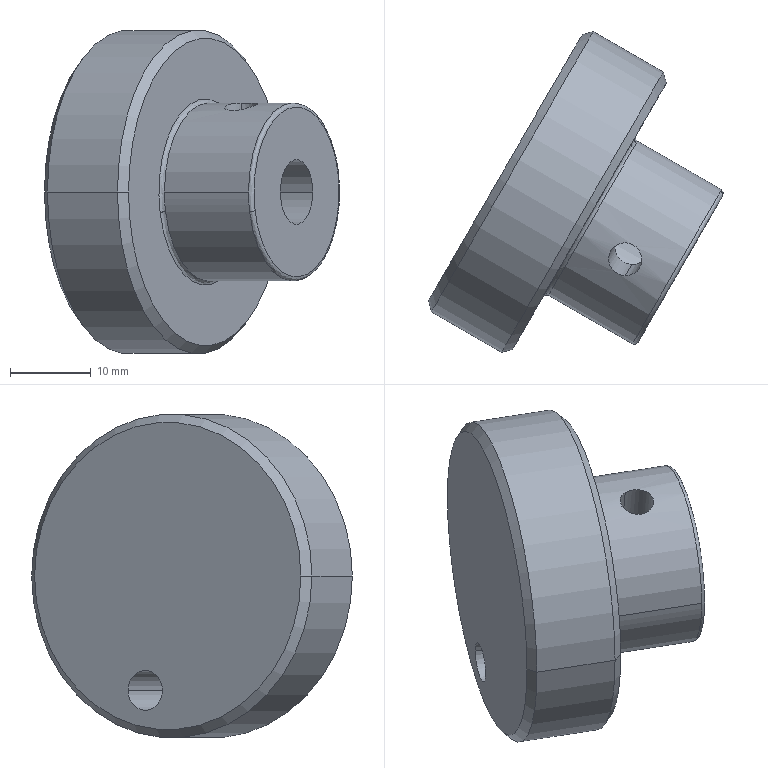Part | SolidWorks | features BaseBody 1 | 1 solid | 26 faces | box 36.468 x 39.641 x 40 mm | volume 18831 mm3 | cylinder 10 | cone 8 | spline 4 | plane 4 | commonest cylinder face diameters 4.134 x2 4.917 x2 8 x2 22 x2 40 x2
STEP:
#1=CARTESIAN_POINT('',(-287.209,1830.124,-1175.566));
#2=VERTEX_POINT('',#1);
#3=CARTESIAN_POINT('',(-298.072,1811.308,-1178.));
#4=VERTEX_POINT('',#3);
#5=CARTESIAN_POINT('',(-292.572,1820.834,-1178.));
#6=DIRECTION('',(0.866,-0.5,0.));
#7=DIRECTION('',(-0.4876,-0.8446,-0.2213));
#8=AXIS2_PLACEMENT_3D('',#5,#6,#7);
#9=CIRCLE('',#8,11.);
#10=EDGE_CURVE('',#2,#4,#9,.T.);
#11=ORIENTED_EDGE('',*,*,#10,.F.);
#12=CARTESIAN_POINT('',(-287.398,1830.796,-1175.455));
#13=VERTEX_POINT('',#12);
#14=CARTESIAN_POINT('',(-286.965,1830.546,-1175.455));
#15=DIRECTION('',(0.1106,0.1916,-0.9752));
#16=DIRECTION('',(0.4876,0.8446,0.2213));
#17=AXIS2_PLACEMENT_3D('',#14,#15,#16);
#18=CIRCLE('',#17,0.5);
#19=EDGE_CURVE('',#2,#13,#18,.T.);
#20=ORIENTED_EDGE('',*,*,#19,.T.);
#21=CARTESIAN_POINT('',(-298.613,1811.372,-1180.545));
#22=VERTEX_POINT('',#21);
#23=CARTESIAN_POINT('',(-287.398,1830.796,-1175.455));
#24=CARTESIAN_POINT('',(-288.143,1829.506,-1168.886));
#25=CARTESIAN_POINT('',(-290.993,1824.57,-1165.294));
#26=CARTESIAN_POINT('',(-294.278,1818.88,-1166.785));
#27=CARTESIAN_POINT('',(-297.562,1813.191,-1168.276));
#28=CARTESIAN_POINT('',(-299.358,1810.081,-1173.975));
#29=CARTESIAN_POINT('',(-298.613,1811.372,-1180.545));
#30=(BOUNDED_CURVE()B_SPLINE_CURVE(3,(#23,#24,#25,#26,#27,#28,#29),.UNSPECIFIED.,.F.,.F.)B_SPLINE_CURVE_WITH_KNOTS((4,3,4),(0.,0.5,1.),.UNSPECIFIED.)CURVE()GEOMETRIC_REPRESENTATION_ITEM()RATIONAL_B_SPLINE_CURVE((1.,0.8047,0.8047,1.,0.8047,0.8047,1.))REPRESENTATION_ITEM(''));
#31=EDGE_CURVE('',#13,#22,#30,.T.);
#32=ORIENTED_EDGE('',*,*,#31,.T.);
#33=CARTESIAN_POINT('',(-297.936,1811.544,-1180.434));
#34=VERTEX_POINT('',#33);
#35=CARTESIAN_POINT('',(-298.18,1811.122,-1180.545));
#36=DIRECTION('',(-0.1106,-0.1916,0.9752));
#37=DIRECTION('',(-0.4876,-0.8446,-0.2213));
#38=AXIS2_PLACEMENT_3D('',#35,#36,#37);
#39=CIRCLE('',#38,0.5);
#40=EDGE_CURVE('',#34,#22,#39,.T.);
#41=ORIENTED_EDGE('',*,*,#40,.F.);
#42=CARTESIAN_POINT('',(-292.572,1820.834,-1178.));
#43=DIRECTION('',(0.866,-0.5,0.));
#44=DIRECTION('',(-0.4876,-0.8446,-0.2213));
#45=AXIS2_PLACEMENT_3D('',#42,#43,#44);
#46=CIRCLE('',#45,11.);
#47=EDGE_CURVE('',#4,#34,#46,.T.);
#48=ORIENTED_EDGE('',*,*,#47,.F.);
#49=EDGE_LOOP('',(#11,#20,#32,#41,#48));
#50=FACE_OUTER_BOUND('',#49,.T.);
#51=CARTESIAN_POINT('',(-297.936,1811.544,-1180.434));
#52=CARTESIAN_POINT('',(-298.649,1810.309,-1174.15));
#53=CARTESIAN_POINT('',(-296.931,1813.284,-1168.698));
#54=CARTESIAN_POINT('',(-293.789,1818.726,-1167.273));
#55=CARTESIAN_POINT('',(-290.647,1824.168,-1165.847));
#56=CARTESIAN_POINT('',(-287.922,1828.889,-1169.282));
#57=CARTESIAN_POINT('',(-287.209,1830.124,-1175.566));
#58=CARTESIAN_POINT('',(-298.19,1811.69,-1180.434));
#59=CARTESIAN_POINT('',(-298.903,1810.456,-1174.15));
#60=CARTESIAN_POINT('',(-297.185,1813.431,-1168.698));
#61=CARTESIAN_POINT('',(-294.043,1818.873,-1167.273));
#62=CARTESIAN_POINT('',(-290.901,1824.315,-1165.847));
#63=CARTESIAN_POINT('',(-288.175,1829.036,-1169.282));
#64=CARTESIAN_POINT('',(-287.462,1830.271,-1175.566));
#65=CARTESIAN_POINT('',(-298.47,1811.619,-1180.48));
#66=CARTESIAN_POINT('',(-299.196,1810.361,-1174.078));
#67=CARTESIAN_POINT('',(-297.446,1813.392,-1168.523));
#68=CARTESIAN_POINT('',(-294.245,1818.936,-1167.071));
#69=CARTESIAN_POINT('',(-291.044,1824.481,-1165.618));
#70=CARTESIAN_POINT('',(-288.267,1829.291,-1169.118));
#71=CARTESIAN_POINT('',(-287.541,1830.549,-1175.52));
#72=CARTESIAN_POINT('',(-298.613,1811.372,-1180.545));
#73=CARTESIAN_POINT('',(-299.358,1810.081,-1173.975));
#74=CARTESIAN_POINT('',(-297.562,1813.191,-1168.276));
#75=CARTESIAN_POINT('',(-294.278,1818.88,-1166.785));
#76=CARTESIAN_POINT('',(-290.993,1824.57,-1165.294));
#77=CARTESIAN_POINT('',(-288.143,1829.506,-1168.886));
#78=CARTESIAN_POINT('',(-287.398,1830.796,-1175.455));
#79=(BOUNDED_SURFACE()B_SPLINE_SURFACE(3,3,((#51,#52,#53,#54,#55,#56,#57),(#58,#59,#60,#61,#62,#63,#64),(#65,#66,#67,#68,#69,#70,#71),(#72,#73,#74,#75,#76,#77,#78)),.UNSPECIFIED.,.F.,.F.,.F.)B_SPLINE_SURFACE_WITH_KNOTS((4,4),(4,3,4),(0.,1.),(0.,0.5,1.),.UNSPECIFIED.)GEOMETRIC_REPRESENTATION_ITEM()RATIONAL_B_SPLINE_SURFACE(((1.,0.8047,0.8047,1.,0.8047,0.8047,1.),(0.8047,0.6476,0.6476,0.8047,0.6476,0.6476,0.8047),(0.8047,0.6476,0.6476,0.8047,0.6476,0.6476,0.8047),(1.,0.8047,0.8047,1.,0.8047,0.8047,1.)))REPRESENTATION_ITEM('')SURFACE());
#80=ADVANCED_FACE('',(#50),#79,.F.);
#81=CARTESIAN_POINT('',(-276.816,1824.124,-1175.566));
#82=VERTEX_POINT('',#81);
#83=CARTESIAN_POINT('',(-276.68,1824.36,-1178.));
#84=VERTEX_POINT('',#83);
#85=CARTESIAN_POINT('',(-282.18,1814.834,-1178.));
#86=DIRECTION('',(-0.866,0.5,0.));
#87=DIRECTION('',(-0.5,-0.866,0.));
#88=AXIS2_PLACEMENT_3D('',#85,#86,#87);
#89=CIRCLE('',#88,11.);
#90=EDGE_CURVE('',#82,#84,#89,.T.);
#91=ORIENTED_EDGE('',*,*,#90,.F.);
#92=CARTESIAN_POINT('',(-276.627,1823.452,-1175.677));
#93=VERTEX_POINT('',#92);
#94=CARTESIAN_POINT('',(-277.06,1823.702,-1175.677));
#95=DIRECTION('',(0.1106,0.1916,-0.9752));
#96=DIRECTION('',(0.4876,0.8446,0.2213));
#97=AXIS2_PLACEMENT_3D('',#94,#95,#96);
#98=CIRCLE('',#97,0.5);
#99=EDGE_CURVE('',#82,#93,#98,.T.);
#100=ORIENTED_EDGE('',*,*,#99,.T.);
#101=CARTESIAN_POINT('',(-286.867,1805.716,-1180.323));
#102=VERTEX_POINT('',#101);
#103=CARTESIAN_POINT('',(-276.627,1823.452,-1175.677));
#104=CARTESIAN_POINT('',(-274.304,1827.476,-1196.156));
#105=CARTESIAN_POINT('',(-284.544,1809.74,-1200.803));
#106=CARTESIAN_POINT('',(-286.867,1805.716,-1180.323));
#107=(BOUNDED_CURVE()B_SPLINE_CURVE(3,(#103,#104,#105,#106),.UNSPECIFIED.,.F.,.F.)B_SPLINE_CURVE_WITH_KNOTS((4,4),(0.,1.),.UNSPECIFIED.)CURVE()GEOMETRIC_REPRESENTATION_ITEM()RATIONAL_B_SPLINE_CURVE((1.,0.3333,0.3333,1.))REPRESENTATION_ITEM(''));
#108=EDGE_CURVE('',#93,#102,#107,.T.);
#109=ORIENTED_EDGE('',*,*,#108,.T.);
#110=CARTESIAN_POINT('',(-287.544,1805.544,-1180.434));
#111=VERTEX_POINT('',#110);
#112=CARTESIAN_POINT('',(-287.3,1805.966,-1180.323));
#113=DIRECTION('',(-0.1106,-0.1916,0.9752));
#114=DIRECTION('',(-0.4876,-0.8446,-0.2213));
#115=AXIS2_PLACEMENT_3D('',#112,#113,#114);
#116=CIRCLE('',#115,0.5);
#117=EDGE_CURVE('',#111,#102,#116,.T.);
#118=ORIENTED_EDGE('',*,*,#117,.F.);
#119=CARTESIAN_POINT('',(-282.18,1814.834,-1178.));
#120=DIRECTION('',(-0.866,0.5,0.));
#121=DIRECTION('',(-0.5,-0.866,0.));
#122=AXIS2_PLACEMENT_3D('',#119,#120,#121);
#123=CIRCLE('',#122,11.);
#124=EDGE_CURVE('',#84,#111,#123,.T.);
#125=ORIENTED_EDGE('',*,*,#124,.F.);
#126=EDGE_LOOP('',(#91,#100,#109,#118,#125));
#127=FACE_OUTER_BOUND('',#126,.T.);
#128=CARTESIAN_POINT('',(-276.816,1824.124,-1175.566));
#129=CARTESIAN_POINT('',(-274.382,1828.34,-1197.021));
#130=CARTESIAN_POINT('',(-285.11,1809.76,-1201.889));
#131=CARTESIAN_POINT('',(-287.544,1805.544,-1180.434));
#132=CARTESIAN_POINT('',(-276.563,1823.978,-1175.566));
#133=CARTESIAN_POINT('',(-274.129,1828.193,-1197.021));
#134=CARTESIAN_POINT('',(-284.856,1809.613,-1201.889));
#135=CARTESIAN_POINT('',(-287.29,1805.397,-1180.434));
#136=CARTESIAN_POINT('',(-276.484,1823.699,-1175.612));
#137=CARTESIAN_POINT('',(-274.096,1827.836,-1196.663));
#138=CARTESIAN_POINT('',(-284.622,1809.605,-1201.439));
#139=CARTESIAN_POINT('',(-287.01,1805.469,-1180.388));
#140=CARTESIAN_POINT('',(-276.627,1823.452,-1175.677));
#141=CARTESIAN_POINT('',(-274.304,1827.476,-1196.156));
#142=CARTESIAN_POINT('',(-284.544,1809.74,-1200.803));
#143=CARTESIAN_POINT('',(-286.867,1805.716,-1180.323));
#144=(BOUNDED_SURFACE()B_SPLINE_SURFACE(3,3,((#128,#129,#130,#131),(#132,#133,#134,#135),(#136,#137,#138,#139),(#140,#141,#142,#143)),.UNSPECIFIED.,.F.,.F.,.F.)B_SPLINE_SURFACE_WITH_KNOTS((4,4),(4,4),(0.,1.),(0.,1.),.UNSPECIFIED.)GEOMETRIC_REPRESENTATION_ITEM()RATIONAL_B_SPLINE_SURFACE(((1.,0.3333,0.3333,1.),(0.8047,0.2682,0.2682,0.8047),(0.8047,0.2682,0.2682,0.8047),(1.,0.3333,0.3333,1.)))REPRESENTATION_ITEM('')SURFACE());
#145=ADVANCED_FACE('',(#127),#144,.T.);
#146=CARTESIAN_POINT('',(-292.77,1827.492,-1192.141));
#147=VERTEX_POINT('',#146);
#148=CARTESIAN_POINT('',(-295.229,1823.233,-1192.141));
#149=VERTEX_POINT('',#148);
#150=CARTESIAN_POINT('',(-293.999,1825.363,-1192.141));
#151=DIRECTION('',(-0.866,0.5,0.));
#152=DIRECTION('',(-0.5,-0.866,0.));
#153=AXIS2_PLACEMENT_3D('',#150,#151,#152);
#154=CIRCLE('',#153,2.459);
#155=EDGE_CURVE('',#147,#149,#154,.T.);
#156=ORIENTED_EDGE('',*,*,#155,.F.);
#157=CARTESIAN_POINT('',(-300.564,1831.992,-1192.141));
#158=VERTEX_POINT('',#157);
#159=CARTESIAN_POINT('',(-300.564,1831.992,-1192.141));
#160=DIRECTION('',(-0.866,0.5,0.));
#161=VECTOR('',#160,1000.);
#162=LINE('',#159,#161);
#163=EDGE_CURVE('',#147,#158,#162,.T.);
#164=ORIENTED_EDGE('',*,*,#163,.T.);
#165=CARTESIAN_POINT('',(-303.023,1827.733,-1192.141));
#166=VERTEX_POINT('',#165);
#167=CARTESIAN_POINT('',(-301.794,1829.863,-1192.141));
#168=DIRECTION('',(-0.866,0.5,0.));
#169=DIRECTION('',(-0.5,-0.866,0.));
#170=AXIS2_PLACEMENT_3D('',#167,#168,#169);
#171=CIRCLE('',#170,2.459);
#172=EDGE_CURVE('',#158,#166,#171,.T.);
#173=ORIENTED_EDGE('',*,*,#172,.T.);
#174=CARTESIAN_POINT('',(-303.023,1827.733,-1192.141));
#175=DIRECTION('',(-0.866,0.5,0.));
#176=VECTOR('',#175,1000.);
#177=LINE('',#174,#176);
#178=EDGE_CURVE('',#149,#166,#177,.T.);
#179=ORIENTED_EDGE('',*,*,#178,.F.);
#180=EDGE_LOOP('',(#156,#164,#173,#179));
#181=FACE_OUTER_BOUND('',#180,.T.);
#182=CARTESIAN_POINT('',(-301.794,1829.863,-1192.141));
#183=DIRECTION('',(-0.866,0.5,0.));
#184=DIRECTION('',(-0.5,-0.866,0.));
#185=AXIS2_PLACEMENT_3D('',#182,#183,#184);
#186=CYLINDRICAL_SURFACE('',#185,2.459);
#187=ADVANCED_FACE('',(#181),#186,.F.);
#188=CARTESIAN_POINT('',(-293.898,1843.538,-1178.));
#189=VERTEX_POINT('',#188);
#190=CARTESIAN_POINT('',(-312.898,1810.63,-1178.));
#191=VERTEX_POINT('',#190);
#192=CARTESIAN_POINT('',(-303.398,1827.084,-1178.));
#193=DIRECTION('',(0.866,-0.5,0.));
#194=DIRECTION('',(0.5,0.866,0.));
#195=AXIS2_PLACEMENT_3D('',#192,#193,#194);
#196=CIRCLE('',#195,19.);
#197=EDGE_CURVE('',#189,#191,#196,.T.);
#198=ORIENTED_EDGE('',*,*,#197,.T.);
#199=CARTESIAN_POINT('',(-312.532,1809.264,-1178.));
#200=VERTEX_POINT('',#199);
#201=CARTESIAN_POINT('',(-312.532,1809.264,-1178.));
#202=DIRECTION('',(0.2588,-0.9659,0.));
#203=VECTOR('',#202,1000.);
#204=LINE('',#201,#203);
#205=EDGE_CURVE('',#191,#200,#204,.T.);
#206=ORIENTED_EDGE('',*,*,#205,.T.);
#207=CARTESIAN_POINT('',(-292.532,1843.905,-1178.));
#208=VERTEX_POINT('',#207);
#209=CARTESIAN_POINT('',(-302.532,1826.584,-1178.));
#210=DIRECTION('',(-0.866,0.5,0.));
#211=DIRECTION('',(0.4876,0.8446,0.2213));
#212=AXIS2_PLACEMENT_3D('',#209,#210,#211);
#213=CIRCLE('',#212,20.);
#214=EDGE_CURVE('',#200,#208,#213,.T.);
#215=ORIENTED_EDGE('',*,*,#214,.T.);
#216=CARTESIAN_POINT('',(-292.532,1843.905,-1178.));
#217=DIRECTION('',(0.9659,0.2588,0.));
#218=VECTOR('',#217,1000.);
#219=LINE('',#216,#218);
#220=EDGE_CURVE('',#189,#208,#219,.T.);
#221=ORIENTED_EDGE('',*,*,#220,.F.);
#222=EDGE_LOOP('',(#198,#206,#215,#221));
#223=FACE_OUTER_BOUND('',#222,.T.);
#224=CARTESIAN_POINT('',(-302.532,1826.584,-1178.));
#225=DIRECTION('',(0.866,-0.5,0.));
#226=DIRECTION('',(0.5,0.866,0.));
#227=AXIS2_PLACEMENT_3D('',#224,#225,#226);
#228=CONICAL_SURFACE('',#227,20.,0.7854);
#229=ADVANCED_FACE('',(#223),#228,.T.);
#230=CARTESIAN_POINT('',(-292.587,1826.809,-1192.141));
#231=VERTEX_POINT('',#230);
#232=CARTESIAN_POINT('',(-294.546,1823.416,-1192.141));
#233=VERTEX_POINT('',#232);
#234=CARTESIAN_POINT('',(-293.566,1825.113,-1192.141));
#235=DIRECTION('',(-0.866,0.5,0.));
#236=DIRECTION('',(-0.5,-0.866,0.));
#237=AXIS2_PLACEMENT_3D('',#234,#235,#236);
#238=CIRCLE('',#237,1.959);
#239=EDGE_CURVE('',#231,#233,#238,.T.);
#240=ORIENTED_EDGE('',*,*,#239,.F.);
#241=CARTESIAN_POINT('',(-292.77,1827.492,-1192.141));
#242=DIRECTION('',(-0.2588,0.9659,0.));
#243=VECTOR('',#242,1000.);
#244=LINE('',#241,#243);
#245=EDGE_CURVE('',#231,#147,#244,.T.);
#246=ORIENTED_EDGE('',*,*,#245,.T.);
#247=ORIENTED_EDGE('',*,*,#155,.T.);
#248=CARTESIAN_POINT('',(-295.229,1823.233,-1192.141));
#249=DIRECTION('',(-0.9659,-0.2588,0.));
#250=VECTOR('',#249,1000.);
#251=LINE('',#248,#250);
#252=EDGE_CURVE('',#233,#149,#251,.T.);
#253=ORIENTED_EDGE('',*,*,#252,.F.);
#254=EDGE_LOOP('',(#240,#246,#247,#253));
#255=FACE_OUTER_BOUND('',#254,.T.);
#256=CARTESIAN_POINT('',(-293.999,1825.363,-1192.141));
#257=DIRECTION('',(-0.866,0.5,0.));
#258=DIRECTION('',(-0.5,-0.866,0.));
#259=AXIS2_PLACEMENT_3D('',#256,#257,#258);
#260=CONICAL_SURFACE('',#259,2.458,0.7854);
#261=ADVANCED_FACE('',(#255),#260,.F.);
#262=CARTESIAN_POINT('',(-303.871,1804.264,-1178.));
#263=VERTEX_POINT('',#262);
#264=CARTESIAN_POINT('',(-283.871,1838.905,-1178.));
#265=VERTEX_POINT('',#264);
#266=CARTESIAN_POINT('',(-293.871,1821.584,-1178.));
#267=DIRECTION('',(-0.866,0.5,0.));
#268=DIRECTION('',(-0.5,-0.866,0.));
#269=AXIS2_PLACEMENT_3D('',#266,#267,#268);
#270=CIRCLE('',#269,20.);
#271=EDGE_CURVE('',#263,#265,#270,.T.);
#272=ORIENTED_EDGE('',*,*,#271,.T.);
#273=CARTESIAN_POINT('',(-293.398,1844.405,-1178.));
#274=DIRECTION('',(-0.866,0.5,0.));
#275=VECTOR('',#274,1000.);
#276=LINE('',#273,#275);
#277=EDGE_CURVE('',#265,#208,#276,.T.);
#278=ORIENTED_EDGE('',*,*,#277,.T.);
#279=ORIENTED_EDGE('',*,*,#214,.F.);
#280=CARTESIAN_POINT('',(-313.398,1809.764,-1178.));
#281=DIRECTION('',(-0.866,0.5,0.));
#282=VECTOR('',#281,1000.);
#283=LINE('',#280,#282);
#284=EDGE_CURVE('',#263,#200,#283,.T.);
#285=ORIENTED_EDGE('',*,*,#284,.F.);
#286=EDGE_LOOP('',(#272,#278,#279,#285));
#287=FACE_OUTER_BOUND('',#286,.T.);
#288=CARTESIAN_POINT('',(-303.398,1827.084,-1178.));
#289=DIRECTION('',(-0.866,0.5,0.));
#290=DIRECTION('',(-0.5,-0.866,0.));
#291=AXIS2_PLACEMENT_3D('',#288,#289,#290);
#292=CYLINDRICAL_SURFACE('',#291,20.);
#293=ADVANCED_FACE('',(#287),#292,.T.);
#294=CARTESIAN_POINT('',(-302.505,1804.63,-1178.));
#295=VERTEX_POINT('',#294);
#296=CARTESIAN_POINT('',(-283.505,1837.538,-1178.));
#297=VERTEX_POINT('',#296);
#298=CARTESIAN_POINT('',(-293.005,1821.084,-1178.));
#299=DIRECTION('',(-0.866,0.5,0.));
#300=DIRECTION('',(-0.5,-0.866,0.));
#301=AXIS2_PLACEMENT_3D('',#298,#299,#300);
#302=CIRCLE('',#301,19.);
#303=EDGE_CURVE('',#295,#297,#302,.T.);
#304=ORIENTED_EDGE('',*,*,#303,.T.);
#305=CARTESIAN_POINT('',(-283.871,1838.905,-1178.));
#306=DIRECTION('',(-0.2588,0.9659,0.));
#307=VECTOR('',#306,1000.);
#308=LINE('',#305,#307);
#309=EDGE_CURVE('',#297,#265,#308,.T.);
#310=ORIENTED_EDGE('',*,*,#309,.T.);
#311=ORIENTED_EDGE('',*,*,#271,.F.);
#312=CARTESIAN_POINT('',(-303.871,1804.264,-1178.));
#313=DIRECTION('',(-0.9659,-0.2588,0.));
#314=VECTOR('',#313,1000.);
#315=LINE('',#312,#314);
#316=EDGE_CURVE('',#295,#263,#315,.T.);
#317=ORIENTED_EDGE('',*,*,#316,.F.);
#318=EDGE_LOOP('',(#304,#310,#311,#317));
#319=FACE_OUTER_BOUND('',#318,.T.);
#320=CARTESIAN_POINT('',(-293.871,1821.584,-1178.));
#321=DIRECTION('',(-0.866,0.5,0.));
#322=DIRECTION('',(-0.5,-0.866,0.));
#323=AXIS2_PLACEMENT_3D('',#320,#321,#322);
#324=CONICAL_SURFACE('',#323,20.,0.7854);
#325=ADVANCED_FACE('',(#319),#324,.T.);
#326=CARTESIAN_POINT('',(-288.577,1813.726,-1167.816));
#327=VERTEX_POINT('',#326);
#328=CARTESIAN_POINT('',(-288.577,1817.783,-1167.019));
#329=VERTEX_POINT('',#328);
#330=CARTESIAN_POINT('',(-288.577,1813.726,-1167.816));
#331=CARTESIAN_POINT('',(-288.71,1813.731,-1167.841));
#332=CARTESIAN_POINT('',(-288.845,1813.749,-1167.863));
#333=CARTESIAN_POINT('',(-289.105,1813.81,-1167.896));
#334=CARTESIAN_POINT('',(-289.233,1813.852,-1167.908));
#335=CARTESIAN_POINT('',(-289.484,1813.961,-1167.922));
#336=CARTESIAN_POINT('',(-289.604,1814.028,-1167.923));
#337=CARTESIAN_POINT('',(-289.828,1814.18,-1167.914));
#338=CARTESIAN_POINT('',(-289.932,1814.265,-1167.905));
#339=CARTESIAN_POINT('',(-290.124,1814.455,-1167.875));
#340=CARTESIAN_POINT('',(-290.211,1814.56,-1167.855));
#341=CARTESIAN_POINT('',(-290.362,1814.779,-1167.808));
#342=CARTESIAN_POINT('',(-290.426,1814.895,-1167.78));
#343=CARTESIAN_POINT('',(-290.532,1815.139,-1167.719));
#344=CARTESIAN_POINT('',(-290.572,1815.264,-1167.685));
#345=CARTESIAN_POINT('',(-290.627,1815.519,-1167.616));
#346=CARTESIAN_POINT('',(-290.641,1815.651,-1167.579));
#347=CARTESIAN_POINT('',(-290.643,1815.912,-1167.505));
#348=CARTESIAN_POINT('',(-290.631,1816.041,-1167.469));
#349=CARTESIAN_POINT('',(-290.58,1816.297,-1167.397));
#350=CARTESIAN_POINT('',(-290.541,1816.425,-1167.362));
#351=CARTESIAN_POINT('',(-290.388,1816.787,-1167.264));
#352=CARTESIAN_POINT('',(-290.233,1817.011,-1167.207));
#353=CARTESIAN_POINT('',(-289.851,1817.381,-1167.118));
#354=CARTESIAN_POINT('',(-289.619,1817.531,-1167.085));
#355=CARTESIAN_POINT('',(-289.244,1817.682,-1167.051));
#356=CARTESIAN_POINT('',(-289.112,1817.721,-1167.042));
#357=CARTESIAN_POINT('',(-288.847,1817.771,-1167.028));
#358=CARTESIAN_POINT('',(-288.713,1817.784,-1167.023));
#359=CARTESIAN_POINT('',(-288.577,1817.783,-1167.019));
#360=B_SPLINE_CURVE_WITH_KNOTS('',3,(#330,#331,#332,#333,#334,#335,#336,#337,#338,#339,#340,#341,#342,#343,#344,#345,#346,#347,#348,#349,#350,#351,#352,#353,#354,#355,#356,#357,#358,#359),.UNSPECIFIED.,.F.,.F.,(4,2,2,2,2,2,2,2,2,2,2,2,2,2,4),(0.0119,0.0123,0.01271,0.01311,0.01352,0.01392,0.01432,0.01473,0.01513,0.01554,0.01594,0.01675,0.01756,0.01797,0.01837),.UNSPECIFIED.);
#361=EDGE_CURVE('',#327,#329,#360,.T.);
#362=ORIENTED_EDGE('',*,*,#361,.T.);
#363=CARTESIAN_POINT('',(-288.577,1817.783,-1167.019));
#364=CARTESIAN_POINT('',(-288.441,1817.782,-1167.015));
#365=CARTESIAN_POINT('',(-288.304,1817.768,-1167.012));
#366=CARTESIAN_POINT('',(-288.04,1817.713,-1167.009));
#367=CARTESIAN_POINT('',(-287.911,1817.673,-1167.008));
#368=CARTESIAN_POINT('',(-287.659,1817.566,-1167.006));
#369=CARTESIAN_POINT('',(-287.538,1817.5,-1167.006));
#370=CARTESIAN_POINT('',(-287.315,1817.346,-1167.007));
#371=CARTESIAN_POINT('',(-287.212,1817.259,-1167.008));
#372=CARTESIAN_POINT('',(-287.024,1817.064,-1167.011));
#373=CARTESIAN_POINT('',(-286.938,1816.956,-1167.013));
#374=CARTESIAN_POINT('',(-286.793,1816.729,-1167.02));
#375=CARTESIAN_POINT('',(-286.731,1816.609,-1167.024));
#376=CARTESIAN_POINT('',(-286.63,1816.354,-1167.037));
#377=CARTESIAN_POINT('',(-286.593,1816.225,-1167.045));
#378=CARTESIAN_POINT('',(-286.544,1815.96,-1167.066));
#379=CARTESIAN_POINT('',(-286.532,1815.824,-1167.079));
#380=CARTESIAN_POINT('',(-286.535,1815.554,-1167.11));
#381=CARTESIAN_POINT('',(-286.549,1815.421,-1167.128));
#382=CARTESIAN_POINT('',(-286.603,1815.159,-1167.17));
#383=CARTESIAN_POINT('',(-286.644,1815.03,-1167.194));
#384=CARTESIAN_POINT('',(-286.799,1814.664,-1167.275));
#385=CARTESIAN_POINT('',(-286.953,1814.442,-1167.34));
#386=CARTESIAN_POINT('',(-287.329,1814.081,-1167.481));
#387=CARTESIAN_POINT('',(-287.556,1813.94,-1167.557));
#388=CARTESIAN_POINT('',(-287.923,1813.804,-1167.663));
#389=CARTESIAN_POINT('',(-288.052,1813.77,-1167.698));
#390=CARTESIAN_POINT('',(-288.312,1813.729,-1167.762));
#391=CARTESIAN_POINT('',(-288.443,1813.721,-1167.791));
#392=CARTESIAN_POINT('',(-288.577,1813.726,-1167.816));
#393=B_SPLINE_CURVE_WITH_KNOTS('',3,(#363,#364,#365,#366,#367,#368,#369,#370,#371,#372,#373,#374,#375,#376,#377,#378,#379,#380,#381,#382,#383,#384,#385,#386,#387,#388,#389,#390,#391,#392),.UNSPECIFIED.,.F.,.F.,(4,2,2,2,2,2,2,2,2,2,2,2,2,2,4),(0.005421,0.005826,0.006231,0.006635,0.00704,0.007445,0.00785,0.008254,0.008659,0.009064,0.009468,0.01028,0.01109,0.01149,0.0119),.UNSPECIFIED.);
#394=EDGE_CURVE('',#329,#327,#393,.T.);
#395=ORIENTED_EDGE('',*,*,#394,.T.);
#396=EDGE_LOOP('',(#362,#395));
#397=FACE_BOUND('',#396,.T.);
#398=CARTESIAN_POINT('',(-287.68,1805.308,-1178.));
#399=VERTEX_POINT('',#398);
#400=CARTESIAN_POINT('',(-282.18,1814.834,-1178.));
#401=DIRECTION('',(-0.866,0.5,0.));
#402=DIRECTION('',(-0.5,-0.866,0.));
#403=AXIS2_PLACEMENT_3D('',#400,#401,#402);
#404=CIRCLE('',#403,11.);
#405=EDGE_CURVE('',#399,#82,#404,.T.);
#406=ORIENTED_EDGE('',*,*,#405,.T.);
#407=ORIENTED_EDGE('',*,*,#90,.T.);
#408=CARTESIAN_POINT('',(-287.072,1830.36,-1178.));
#409=VERTEX_POINT('',#408);
#410=CARTESIAN_POINT('',(-297.898,1836.61,-1178.));
#411=DIRECTION('',(-0.866,0.5,0.));
#412=VECTOR('',#411,1000.);
#413=LINE('',#410,#412);
#414=EDGE_CURVE('',#84,#409,#413,.T.);
#415=ORIENTED_EDGE('',*,*,#414,.T.);
#416=CARTESIAN_POINT('',(-292.572,1820.834,-1178.));
#417=DIRECTION('',(0.866,-0.5,0.));
#418=DIRECTION('',(-0.4876,-0.8446,-0.2213));
#419=AXIS2_PLACEMENT_3D('',#416,#417,#418);
#420=CIRCLE('',#419,11.);
#421=EDGE_CURVE('',#409,#2,#420,.T.);
#422=ORIENTED_EDGE('',*,*,#421,.T.);
#423=ORIENTED_EDGE('',*,*,#10,.T.);
#424=CARTESIAN_POINT('',(-308.898,1817.558,-1178.));
#425=DIRECTION('',(-0.866,0.5,0.));
#426=VECTOR('',#425,1000.);
#427=LINE('',#424,#426);
#428=EDGE_CURVE('',#399,#4,#427,.T.);
#429=ORIENTED_EDGE('',*,*,#428,.F.);
#430=EDGE_LOOP('',(#406,#407,#415,#422,#423,#429));
#431=FACE_OUTER_BOUND('',#430,.T.);
#432=CARTESIAN_POINT('',(-303.398,1827.084,-1178.));
#433=DIRECTION('',(-0.866,0.5,0.));
#434=DIRECTION('',(-0.5,-0.866,0.));
#435=AXIS2_PLACEMENT_3D('',#432,#433,#434);
#436=CYLINDRICAL_SURFACE('',#435,11.);
#437=ADVANCED_FACE('',(#397,#431),#436,.T.);
#438=CARTESIAN_POINT('',(-287.771,1819.178,-1174.118));
#439=VERTEX_POINT('',#438);
#440=CARTESIAN_POINT('',(-287.771,1815.121,-1174.916));
#441=VERTEX_POINT('',#440);
#442=CARTESIAN_POINT('',(-287.771,1819.178,-1174.118));
#443=CARTESIAN_POINT('',(-287.908,1819.174,-1174.101));
#444=CARTESIAN_POINT('',(-288.045,1819.157,-1174.082));
#445=CARTESIAN_POINT('',(-288.312,1819.099,-1174.048));
#446=CARTESIAN_POINT('',(-288.442,1819.057,-1174.033));
#447=CARTESIAN_POINT('',(-288.696,1818.95,-1174.01));
#448=CARTESIAN_POINT('',(-288.819,1818.885,-1174.003));
#449=CARTESIAN_POINT('',(-289.047,1818.734,-1173.999));
#450=CARTESIAN_POINT('',(-289.155,1818.649,-1174.002));
#451=CARTESIAN_POINT('',(-289.354,1818.456,-1174.023));
#452=CARTESIAN_POINT('',(-289.443,1818.353,-1174.041));
#453=CARTESIAN_POINT('',(-289.596,1818.131,-1174.09));
#454=CARTESIAN_POINT('',(-289.662,1818.012,-1174.122));
#455=CARTESIAN_POINT('',(-289.766,1817.768,-1174.199));
#456=CARTESIAN_POINT('',(-289.804,1817.644,-1174.243));
#457=CARTESIAN_POINT('',(-289.852,1817.39,-1174.342));
#458=CARTESIAN_POINT('',(-289.862,1817.262,-1174.396));
#459=CARTESIAN_POINT('',(-289.855,1817.01,-1174.507));
#460=CARTESIAN_POINT('',(-289.838,1816.885,-1174.565));
#461=CARTESIAN_POINT('',(-289.779,1816.641,-1174.681));
#462=CARTESIAN_POINT('',(-289.737,1816.523,-1174.737));
#463=CARTESIAN_POINT('',(-289.629,1816.293,-1174.845));
#464=CARTESIAN_POINT('',(-289.563,1816.181,-1174.897));
#465=CARTESIAN_POINT('',(-289.41,1815.971,-1174.985));
#466=CARTESIAN_POINT('',(-289.323,1815.872,-1175.023));
#467=CARTESIAN_POINT('',(-289.031,1815.592,-1175.112));
#468=CARTESIAN_POINT('',(-288.794,1815.432,-1175.132));
#469=CARTESIAN_POINT('',(-288.295,1815.208,-1175.08));
#470=CARTESIAN_POINT('',(-288.03,1815.14,-1175.009));
#471=CARTESIAN_POINT('',(-287.771,1815.121,-1174.916));
#472=B_SPLINE_CURVE_WITH_KNOTS('',3,(#442,#443,#444,#445,#446,#447,#448,#449,#450,#451,#452,#453,#454,#455,#456,#457,#458,#459,#460,#461,#462,#463,#464,#465,#466,#467,#468,#469,#470,#471),.UNSPECIFIED.,.F.,.F.,(4,2,2,2,2,2,2,2,2,2,2,2,2,2,4),(0.001068,0.001479,0.00189,0.002301,0.002713,0.003124,0.003535,0.003946,0.004357,0.004768,0.005179,0.005591,0.006002,0.006824,0.007646),.UNSPECIFIED.);
#473=EDGE_CURVE('',#439,#441,#472,.T.);
#474=ORIENTED_EDGE('',*,*,#473,.F.);
#475=CARTESIAN_POINT('',(-288.593,1817.754,-1166.874));
#476=DIRECTION('',(-0.1106,-0.1916,0.9752));
#477=VECTOR('',#476,1000.);
#478=LINE('',#475,#477);
#479=EDGE_CURVE('',#439,#329,#478,.T.);
#480=ORIENTED_EDGE('',*,*,#479,.T.);
#481=ORIENTED_EDGE('',*,*,#361,.F.);
#482=CARTESIAN_POINT('',(-288.593,1813.698,-1167.671));
#483=DIRECTION('',(-0.1106,-0.1916,0.9752));
#484=VECTOR('',#483,1000.);
#485=LINE('',#482,#484);
#486=EDGE_CURVE('',#441,#327,#485,.T.);
#487=ORIENTED_EDGE('',*,*,#486,.F.);
#488=EDGE_LOOP('',(#474,#480,#481,#487));
#489=FACE_OUTER_BOUND('',#488,.T.);
#490=CARTESIAN_POINT('',(-288.593,1815.726,-1167.273));
#491=DIRECTION('',(-0.1106,-0.1916,0.9752));
#492=DIRECTION('',(0.,-0.9812,-0.1928));
#493=AXIS2_PLACEMENT_3D('',#490,#491,#492);
#494=CYLINDRICAL_SURFACE('',#493,2.067);
#495=ADVANCED_FACE('',(#489),#494,.F.);
#496=CARTESIAN_POINT('',(-296.737,1818.62,-1178.));
#497=VERTEX_POINT('',#496);
#498=CARTESIAN_POINT('',(-292.737,1825.548,-1178.));
#499=VERTEX_POINT('',#498);
#500=CARTESIAN_POINT('',(-294.737,1822.084,-1178.));
#501=DIRECTION('',(0.866,-0.5,0.));
#502=DIRECTION('',(0.5,0.866,0.));
#503=AXIS2_PLACEMENT_3D('',#500,#501,#502);
#504=CIRCLE('',#503,4.);
#505=EDGE_CURVE('',#497,#499,#504,.T.);
#506=ORIENTED_EDGE('',*,*,#505,.F.);
#507=CARTESIAN_POINT('',(-283.747,1811.12,-1178.));
#508=VERTEX_POINT('',#507);
#509=CARTESIAN_POINT('',(-283.747,1811.12,-1178.));
#510=DIRECTION('',(0.866,-0.5,0.));
#511=VECTOR('',#510,1000.);
#512=LINE('',#509,#511);
#513=EDGE_CURVE('',#497,#508,#512,.T.);
#514=ORIENTED_EDGE('',*,*,#513,.T.);
#515=CARTESIAN_POINT('',(-279.747,1818.048,-1178.));
#516=VERTEX_POINT('',#515);
#517=CARTESIAN_POINT('',(-281.747,1814.584,-1178.));
#518=DIRECTION('',(-0.866,0.5,0.));
#519=DIRECTION('',(0.5,0.866,0.));
#520=AXIS2_PLACEMENT_3D('',#517,#518,#519);
#521=CIRCLE('',#520,4.);
#522=EDGE_CURVE('',#516,#508,#521,.T.);
#523=ORIENTED_EDGE('',*,*,#522,.F.);
#524=CARTESIAN_POINT('',(-279.747,1818.048,-1178.));
#525=DIRECTION('',(0.866,-0.5,0.));
#526=VECTOR('',#525,1000.);
#527=LINE('',#524,#526);
#528=EDGE_CURVE('',#499,#516,#527,.T.);
#529=ORIENTED_EDGE('',*,*,#528,.F.);
#530=EDGE_LOOP('',(#506,#514,#523,#529));
#531=FACE_OUTER_BOUND('',#530,.T.);
#532=CARTESIAN_POINT('',(-281.747,1814.584,-1178.));
#533=DIRECTION('',(0.866,-0.5,0.));
#534=DIRECTION('',(0.5,0.866,0.));
#535=AXIS2_PLACEMENT_3D('',#532,#533,#534);
#536=CYLINDRICAL_SURFACE('',#535,4.);
#537=ADVANCED_FACE('',(#531),#536,.F.);
#538=CARTESIAN_POINT('',(-296.819,1823.286,-1178.));
#539=VERTEX_POINT('',#538);
#540=CARTESIAN_POINT('',(-292.737,1825.548,-1178.));
#541=DIRECTION('',(0.8746,0.4848,0.));
#542=VECTOR('',#541,1000.);
#543=LINE('',#540,#542);
#544=EDGE_CURVE('',#539,#499,#543,.T.);
#545=ORIENTED_EDGE('',*,*,#544,.F.);
#546=CARTESIAN_POINT('',(-296.737,1818.62,-1178.));
#547=DIRECTION('',(0.01745,-0.9998,0.));
#548=VECTOR('',#547,1000.);
#549=LINE('',#546,#548);
#550=EDGE_CURVE('',#539,#497,#549,.T.);
#551=ORIENTED_EDGE('',*,*,#550,.T.);
#552=ORIENTED_EDGE('',*,*,#505,.T.);
#553=EDGE_LOOP('',(#545,#551,#552));
#554=FACE_OUTER_BOUND('',#553,.T.);
#555=CARTESIAN_POINT('',(-294.737,1822.084,-1178.));
#556=DIRECTION('',(0.866,-0.5,0.));
#557=DIRECTION('',(0.5,0.866,0.));
#558=AXIS2_PLACEMENT_3D('',#555,#556,#557);
#559=CONICAL_SURFACE('',#558,4.,1.03);
#560=ADVANCED_FACE('',(#554),#559,.F.);
#561=CARTESIAN_POINT('',(-301.794,1829.863,-1192.141));
#562=DIRECTION('',(-0.866,0.5,0.));
#563=DIRECTION('',(-0.5,-0.866,0.));
#564=AXIS2_PLACEMENT_3D('',#561,#562,#563);
#565=CIRCLE('',#564,2.459);
#566=EDGE_CURVE('',#166,#158,#565,.T.);
#567=ORIENTED_EDGE('',*,*,#566,.F.);
#568=ORIENTED_EDGE('',*,*,#172,.F.);
#569=EDGE_LOOP('',(#567,#568));
#570=FACE_BOUND('',#569,.T.);
#571=ORIENTED_EDGE('',*,*,#197,.F.);
#572=CARTESIAN_POINT('',(-303.398,1827.084,-1178.));
#573=DIRECTION('',(0.866,-0.5,0.));
#574=DIRECTION('',(0.5,0.866,0.));
#575=AXIS2_PLACEMENT_3D('',#572,#573,#574);
#576=CIRCLE('',#575,19.);
#577=EDGE_CURVE('',#191,#189,#576,.T.);
#578=ORIENTED_EDGE('',*,*,#577,.F.);
#579=EDGE_LOOP('',(#571,#578));
#580=FACE_OUTER_BOUND('',#579,.T.);
#581=CARTESIAN_POINT('',(-305.5,1823.443,-1159.471));
#582=DIRECTION('',(0.866,-0.5,0.));
#583=DIRECTION('',(0.5,0.866,0.));
#584=AXIS2_PLACEMENT_3D('',#581,#582,#583);
#585=PLANE('',#584);
#586=ADVANCED_FACE('',(#570,#580),#585,.F.);
#587=ORIENTED_EDGE('',*,*,#163,.F.);
#588=CARTESIAN_POINT('',(-293.999,1825.363,-1192.141));
#589=DIRECTION('',(-0.866,0.5,0.));
#590=DIRECTION('',(-0.5,-0.866,0.));
#591=AXIS2_PLACEMENT_3D('',#588,#589,#590);
#592=CIRCLE('',#591,2.459);
#593=EDGE_CURVE('',#149,#147,#592,.T.);
#594=ORIENTED_EDGE('',*,*,#593,.F.);
#595=ORIENTED_EDGE('',*,*,#178,.T.);
#596=ORIENTED_EDGE('',*,*,#566,.T.);
#597=EDGE_LOOP('',(#587,#594,#595,#596));
#598=FACE_OUTER_BOUND('',#597,.T.);
#599=CARTESIAN_POINT('',(-301.794,1829.863,-1192.141));
#600=DIRECTION('',(-0.866,0.5,0.));
#601=DIRECTION('',(-0.5,-0.866,0.));
#602=AXIS2_PLACEMENT_3D('',#599,#600,#601);
#603=CYLINDRICAL_SURFACE('',#602,2.459);
#604=ADVANCED_FACE('',(#598),#603,.F.);
#605=ORIENTED_EDGE('',*,*,#205,.F.);
#606=ORIENTED_EDGE('',*,*,#577,.T.);
#607=ORIENTED_EDGE('',*,*,#220,.T.);
#608=CARTESIAN_POINT('',(-302.532,1826.584,-1178.));
#609=DIRECTION('',(-0.866,0.5,0.));
#610=DIRECTION('',(0.4876,0.8446,0.2213));
#611=AXIS2_PLACEMENT_3D('',#608,#609,#610);
#612=CIRCLE('',#611,20.);
#613=EDGE_CURVE('',#208,#200,#612,.T.);
#614=ORIENTED_EDGE('',*,*,#613,.T.);
#615=EDGE_LOOP('',(#605,#606,#607,#614));
#616=FACE_OUTER_BOUND('',#615,.T.);
#617=CARTESIAN_POINT('',(-302.532,1826.584,-1178.));
#618=DIRECTION('',(0.866,-0.5,0.));
#619=DIRECTION('',(0.5,0.866,0.));
#620=AXIS2_PLACEMENT_3D('',#617,#618,#619);
#621=CONICAL_SURFACE('',#620,20.,0.7854);
#622=ADVANCED_FACE('',(#616),#621,.T.);
#623=ORIENTED_EDGE('',*,*,#245,.F.);
#624=CARTESIAN_POINT('',(-293.566,1825.113,-1192.141));
#625=DIRECTION('',(-0.866,0.5,0.));
#626=DIRECTION('',(-0.5,-0.866,0.));
#627=AXIS2_PLACEMENT_3D('',#624,#625,#626);
#628=CIRCLE('',#627,1.959);
#629=EDGE_CURVE('',#233,#231,#628,.T.);
#630=ORIENTED_EDGE('',*,*,#629,.F.);
#631=ORIENTED_EDGE('',*,*,#252,.T.);
#632=ORIENTED_EDGE('',*,*,#593,.T.);
#633=EDGE_LOOP('',(#623,#630,#631,#632));
#634=FACE_OUTER_BOUND('',#633,.T.);
#635=CARTESIAN_POINT('',(-293.999,1825.363,-1192.141));
#636=DIRECTION('',(-0.866,0.5,0.));
#637=DIRECTION('',(-0.5,-0.866,0.));
#638=AXIS2_PLACEMENT_3D('',#635,#636,#637);
#639=CONICAL_SURFACE('',#638,2.458,0.7854);
#640=ADVANCED_FACE('',(#634),#639,.F.);
#641=ORIENTED_EDGE('',*,*,#277,.F.);
#642=CARTESIAN_POINT('',(-293.871,1821.584,-1178.));
#643=DIRECTION('',(-0.866,0.5,0.));
#644=DIRECTION('',(-0.5,-0.866,0.));
#645=AXIS2_PLACEMENT_3D('',#642,#643,#644);
#646=CIRCLE('',#645,20.);
#647=EDGE_CURVE('',#265,#263,#646,.T.);
#648=ORIENTED_EDGE('',*,*,#647,.T.);
#649=ORIENTED_EDGE('',*,*,#284,.T.);
#650=ORIENTED_EDGE('',*,*,#613,.F.);
#651=EDGE_LOOP('',(#641,#648,#649,#650));
#652=FACE_OUTER_BOUND('',#651,.T.);
#653=CARTESIAN_POINT('',(-303.398,1827.084,-1178.));
#654=DIRECTION('',(-0.866,0.5,0.));
#655=DIRECTION('',(-0.5,-0.866,0.));
#656=AXIS2_PLACEMENT_3D('',#653,#654,#655);
#657=CYLINDRICAL_SURFACE('',#656,20.);
#658=ADVANCED_FACE('',(#652),#657,.T.);
#659=ORIENTED_EDGE('',*,*,#629,.T.);
#660=ORIENTED_EDGE('',*,*,#239,.T.);
#661=EDGE_LOOP('',(#659,#660));
#662=FACE_OUTER_BOUND('',#661,.T.);
#663=CARTESIAN_POINT('',(-293.566,1825.113,-1192.141));
#664=DIRECTION('',(0.866,-0.5,0.));
#665=DIRECTION('',(0.5,0.866,0.));
#666=AXIS2_PLACEMENT_3D('',#663,#664,#665);
#667=PLANE('',#666);
#668=ADVANCED_FACE('',(#662),#667,.F.);
#669=ORIENTED_EDGE('',*,*,#309,.F.);
#670=CARTESIAN_POINT('',(-293.005,1821.084,-1178.));
#671=DIRECTION('',(-0.866,0.5,0.));
#672=DIRECTION('',(-0.5,-0.866,0.));
#673=AXIS2_PLACEMENT_3D('',#670,#671,#672);
#674=CIRCLE('',#673,19.);
#675=EDGE_CURVE('',#297,#295,#674,.T.);
#676=ORIENTED_EDGE('',*,*,#675,.T.);
#677=ORIENTED_EDGE('',*,*,#316,.T.);
#678=ORIENTED_EDGE('',*,*,#647,.F.);
#679=EDGE_LOOP('',(#669,#676,#677,#678));
#680=FACE_OUTER_BOUND('',#679,.T.);
#681=CARTESIAN_POINT('',(-293.871,1821.584,-1178.));
#682=DIRECTION('',(-0.866,0.5,0.));
#683=DIRECTION('',(-0.5,-0.866,0.));
#684=AXIS2_PLACEMENT_3D('',#681,#682,#683);
#685=CONICAL_SURFACE('',#684,20.,0.7854);
#686=ADVANCED_FACE('',(#680),#685,.T.);
#687=ORIENTED_EDGE('',*,*,#31,.F.);
#688=CARTESIAN_POINT('',(-298.613,1811.372,-1180.545));
#689=CARTESIAN_POINT('',(-296.068,1815.779,-1202.974));
#690=CARTESIAN_POINT('',(-284.853,1835.204,-1197.885));
#691=CARTESIAN_POINT('',(-287.398,1830.796,-1175.455));
#692=(BOUNDED_CURVE()B_SPLINE_CURVE(3,(#688,#689,#690,#691),.UNSPECIFIED.,.F.,.T.)B_SPLINE_CURVE_WITH_KNOTS((4,4),(0.,1.),.UNSPECIFIED.)CURVE()GEOMETRIC_REPRESENTATION_ITEM()RATIONAL_B_SPLINE_CURVE((1.,0.3333,0.3333,1.))REPRESENTATION_ITEM(''));
#693=EDGE_CURVE('',#22,#13,#692,.T.);
#694=ORIENTED_EDGE('',*,*,#693,.F.);
#695=EDGE_LOOP('',(#687,#694));
#696=FACE_BOUND('',#695,.T.);
#697=ORIENTED_EDGE('',*,*,#303,.F.);
#698=ORIENTED_EDGE('',*,*,#675,.F.);
#699=EDGE_LOOP('',(#697,#698));
#700=FACE_OUTER_BOUND('',#699,.T.);
#701=CARTESIAN_POINT('',(-294.222,1818.976,-1167.273));
#702=DIRECTION('',(-0.866,0.5,0.));
#703=DIRECTION('',(-0.5,-0.866,0.));
#704=AXIS2_PLACEMENT_3D('',#701,#702,#703);
#705=PLANE('',#704);
#706=ADVANCED_FACE('',(#696,#700),#705,.F.);
#707=ORIENTED_EDGE('',*,*,#19,.F.);
#708=ORIENTED_EDGE('',*,*,#421,.F.);
#709=CARTESIAN_POINT('',(-292.572,1820.834,-1178.));
#710=DIRECTION('',(0.866,-0.5,0.));
#711=DIRECTION('',(-0.4876,-0.8446,-0.2213));
#712=AXIS2_PLACEMENT_3D('',#709,#710,#711);
#713=CIRCLE('',#712,11.);
#714=EDGE_CURVE('',#34,#409,#713,.T.);
#715=ORIENTED_EDGE('',*,*,#714,.F.);
#716=ORIENTED_EDGE('',*,*,#40,.T.);
#717=ORIENTED_EDGE('',*,*,#693,.T.);
#718=EDGE_LOOP('',(#707,#708,#715,#716,#717));
#719=FACE_OUTER_BOUND('',#718,.T.);
#720=CARTESIAN_POINT('',(-287.209,1830.124,-1175.566));
#721=CARTESIAN_POINT('',(-284.775,1834.34,-1197.021));
#722=CARTESIAN_POINT('',(-295.502,1815.76,-1201.889));
#723=CARTESIAN_POINT('',(-297.936,1811.544,-1180.434));
#724=CARTESIAN_POINT('',(-287.462,1830.271,-1175.566));
#725=CARTESIAN_POINT('',(-285.028,1834.486,-1197.021));
#726=CARTESIAN_POINT('',(-295.756,1815.906,-1201.889));
#727=CARTESIAN_POINT('',(-298.19,1811.69,-1180.434));
#728=CARTESIAN_POINT('',(-287.541,1830.549,-1175.52));
#729=CARTESIAN_POINT('',(-285.061,1834.844,-1197.379));
#730=CARTESIAN_POINT('',(-295.99,1815.914,-1202.338));
#731=CARTESIAN_POINT('',(-298.47,1811.619,-1180.48));
#732=CARTESIAN_POINT('',(-287.398,1830.796,-1175.455));
#733=CARTESIAN_POINT('',(-284.853,1835.204,-1197.885));
#734=CARTESIAN_POINT('',(-296.068,1815.779,-1202.974));
#735=CARTESIAN_POINT('',(-298.613,1811.372,-1180.545));
#736=(BOUNDED_SURFACE()B_SPLINE_SURFACE(3,3,((#720,#721,#722,#723),(#724,#725,#726,#727),(#728,#729,#730,#731),(#732,#733,#734,#735)),.UNSPECIFIED.,.F.,.F.,.F.)B_SPLINE_SURFACE_WITH_KNOTS((4,4),(4,4),(0.,1.),(0.,1.),.UNSPECIFIED.)GEOMETRIC_REPRESENTATION_ITEM()RATIONAL_B_SPLINE_SURFACE(((1.,0.3333,0.3333,1.),(0.8047,0.2682,0.2682,0.8047),(0.8047,0.2682,0.2682,0.8047),(1.,0.3333,0.3333,1.)))REPRESENTATION_ITEM('')SURFACE());
#737=ADVANCED_FACE('',(#719),#736,.F.);
#738=ORIENTED_EDGE('',*,*,#414,.F.);
#739=ORIENTED_EDGE('',*,*,#124,.T.);
#740=CARTESIAN_POINT('',(-282.18,1814.834,-1178.));
#741=DIRECTION('',(-0.866,0.5,0.));
#742=DIRECTION('',(-0.5,-0.866,0.));
#743=AXIS2_PLACEMENT_3D('',#740,#741,#742);
#744=CIRCLE('',#743,11.);
#745=EDGE_CURVE('',#111,#399,#744,.T.);
#746=ORIENTED_EDGE('',*,*,#745,.T.);
#747=ORIENTED_EDGE('',*,*,#428,.T.);
#748=ORIENTED_EDGE('',*,*,#47,.T.);
#749=ORIENTED_EDGE('',*,*,#714,.T.);
#750=EDGE_LOOP('',(#738,#739,#746,#747,#748,#749));
#751=FACE_OUTER_BOUND('',#750,.T.);
#752=CARTESIAN_POINT('',(-303.398,1827.084,-1178.));
#753=DIRECTION('',(-0.866,0.5,0.));
#754=DIRECTION('',(-0.5,-0.866,0.));
#755=AXIS2_PLACEMENT_3D('',#752,#753,#754);
#756=CYLINDRICAL_SURFACE('',#755,11.);
#757=ADVANCED_FACE('',(#751),#756,.T.);
#758=ORIENTED_EDGE('',*,*,#99,.F.);
#759=ORIENTED_EDGE('',*,*,#405,.F.);
#760=ORIENTED_EDGE('',*,*,#745,.F.);
#761=ORIENTED_EDGE('',*,*,#117,.T.);
#762=CARTESIAN_POINT('',(-286.867,1805.716,-1180.323));
#763=CARTESIAN_POINT('',(-287.547,1804.538,-1174.325));
#764=CARTESIAN_POINT('',(-285.908,1807.377,-1169.121));
#765=CARTESIAN_POINT('',(-282.909,1812.572,-1167.76));
#766=CARTESIAN_POINT('',(-279.91,1817.767,-1166.399));
#767=CARTESIAN_POINT('',(-277.308,1822.273,-1169.678));
#768=CARTESIAN_POINT('',(-276.627,1823.452,-1175.677));
#769=(BOUNDED_CURVE()B_SPLINE_CURVE(3,(#762,#763,#764,#765,#766,#767,#768),.UNSPECIFIED.,.F.,.T.)B_SPLINE_CURVE_WITH_KNOTS((4,3,4),(0.,0.5,1.),.UNSPECIFIED.)CURVE()GEOMETRIC_REPRESENTATION_ITEM()RATIONAL_B_SPLINE_CURVE((1.,0.8047,0.8047,1.,0.8047,0.8047,1.))REPRESENTATION_ITEM(''));
#770=EDGE_CURVE('',#102,#93,#769,.T.);
#771=ORIENTED_EDGE('',*,*,#770,.T.);
#772=EDGE_LOOP('',(#758,#759,#760,#761,#771));
#773=FACE_OUTER_BOUND('',#772,.T.);
#774=CARTESIAN_POINT('',(-287.544,1805.544,-1180.434));
#775=CARTESIAN_POINT('',(-288.257,1804.309,-1174.15));
#776=CARTESIAN_POINT('',(-286.539,1807.284,-1168.698));
#777=CARTESIAN_POINT('',(-283.397,1812.726,-1167.273));
#778=CARTESIAN_POINT('',(-280.255,1818.168,-1165.847));
#779=CARTESIAN_POINT('',(-277.529,1822.889,-1169.282));
#780=CARTESIAN_POINT('',(-276.816,1824.124,-1175.566));
#781=CARTESIAN_POINT('',(-287.29,1805.397,-1180.434));
#782=CARTESIAN_POINT('',(-288.003,1804.163,-1174.15));
#783=CARTESIAN_POINT('',(-286.285,1807.138,-1168.698));
#784=CARTESIAN_POINT('',(-283.143,1812.58,-1167.273));
#785=CARTESIAN_POINT('',(-280.001,1818.022,-1165.847));
#786=CARTESIAN_POINT('',(-277.276,1822.743,-1169.282));
#787=CARTESIAN_POINT('',(-276.563,1823.978,-1175.566));
#788=CARTESIAN_POINT('',(-287.01,1805.469,-1180.388));
#789=CARTESIAN_POINT('',(-287.709,1804.257,-1174.222));
#790=CARTESIAN_POINT('',(-286.024,1807.176,-1168.874));
#791=CARTESIAN_POINT('',(-282.941,1812.516,-1167.475));
#792=CARTESIAN_POINT('',(-279.858,1817.855,-1166.076));
#793=CARTESIAN_POINT('',(-277.184,1822.488,-1169.446));
#794=CARTESIAN_POINT('',(-276.484,1823.699,-1175.612));
#795=CARTESIAN_POINT('',(-286.867,1805.716,-1180.323));
#796=CARTESIAN_POINT('',(-287.547,1804.538,-1174.325));
#797=CARTESIAN_POINT('',(-285.908,1807.377,-1169.121));
#798=CARTESIAN_POINT('',(-282.909,1812.572,-1167.76));
#799=CARTESIAN_POINT('',(-279.91,1817.767,-1166.399));
#800=CARTESIAN_POINT('',(-277.308,1822.273,-1169.678));
#801=CARTESIAN_POINT('',(-276.627,1823.452,-1175.677));
#802=(BOUNDED_SURFACE()B_SPLINE_SURFACE(3,3,((#774,#775,#776,#777,#778,#779,#780),(#781,#782,#783,#784,#785,#786,#787),(#788,#789,#790,#791,#792,#793,#794),(#795,#796,#797,#798,#799,#800,#801)),.UNSPECIFIED.,.F.,.F.,.F.)B_SPLINE_SURFACE_WITH_KNOTS((4,4),(4,3,4),(0.,1.),(0.,0.5,1.),.UNSPECIFIED.)GEOMETRIC_REPRESENTATION_ITEM()RATIONAL_B_SPLINE_SURFACE(((1.,0.8047,0.8047,1.,0.8047,0.8047,1.),(0.8047,0.6476,0.6476,0.8047,0.6476,0.6476,0.8047),(0.8047,0.6476,0.6476,0.8047,0.6476,0.6476,0.8047),(1.,0.8047,0.8047,1.,0.8047,0.8047,1.)))REPRESENTATION_ITEM('')SURFACE());
#803=ADVANCED_FACE('',(#773),#802,.T.);
#804=ORIENTED_EDGE('',*,*,#479,.F.);
#805=CARTESIAN_POINT('',(-287.771,1815.121,-1174.916));
#806=CARTESIAN_POINT('',(-287.642,1815.112,-1174.869));
#807=CARTESIAN_POINT('',(-287.513,1815.115,-1174.816));
#808=CARTESIAN_POINT('',(-287.262,1815.146,-1174.706));
#809=CARTESIAN_POINT('',(-287.14,1815.173,-1174.649));
#810=CARTESIAN_POINT('',(-286.902,1815.253,-1174.533));
#811=CARTESIAN_POINT('',(-286.787,1815.305,-1174.475));
#812=CARTESIAN_POINT('',(-286.571,1815.434,-1174.366));
#813=CARTESIAN_POINT('',(-286.469,1815.509,-1174.314));
#814=CARTESIAN_POINT('',(-286.278,1815.688,-1174.218));
#815=CARTESIAN_POINT('',(-286.193,1815.786,-1174.176));
#816=CARTESIAN_POINT('',(-286.041,1816.003,-1174.104));
#817=CARTESIAN_POINT('',(-285.975,1816.123,-1174.075));
#818=CARTESIAN_POINT('',(-285.868,1816.374,-1174.03));
#819=CARTESIAN_POINT('',(-285.827,1816.504,-1174.016));
#820=CARTESIAN_POINT('',(-285.769,1816.774,-1173.999));
#821=CARTESIAN_POINT('',(-285.753,1816.913,-1173.998));
#822=CARTESIAN_POINT('',(-285.747,1817.187,-1174.006));
#823=CARTESIAN_POINT('',(-285.756,1817.326,-1174.016));
#824=CARTESIAN_POINT('',(-285.799,1817.598,-1174.041));
#825=CARTESIAN_POINT('',(-285.833,1817.73,-1174.058));
#826=CARTESIAN_POINT('',(-285.925,1817.988,-1174.092));
#827=CARTESIAN_POINT('',(-285.984,1818.114,-1174.111));
#828=CARTESIAN_POINT('',(-286.122,1818.348,-1174.146));
#829=CARTESIAN_POINT('',(-286.203,1818.458,-1174.162));
#830=CARTESIAN_POINT('',(-286.481,1818.763,-1174.2));
#831=CARTESIAN_POINT('',(-286.715,1818.928,-1174.209));
#832=CARTESIAN_POINT('',(-287.222,1819.137,-1174.186));
#833=CARTESIAN_POINT('',(-287.499,1819.185,-1174.154));
#834=CARTESIAN_POINT('',(-287.771,1819.178,-1174.118));
#835=B_SPLINE_CURVE_WITH_KNOTS('',3,(#805,#806,#807,#808,#809,#810,#811,#812,#813,#814,#815,#816,#817,#818,#819,#820,#821,#822,#823,#824,#825,#826,#827,#828,#829,#830,#831,#832,#833,#834),.UNSPECIFIED.,.F.,.F.,(4,2,2,2,2,2,2,2,2,2,2,2,2,2,4),(0.007646,0.008057,0.008468,0.008879,0.00929,0.009701,0.01011,0.01052,0.01093,0.01134,0.01176,0.01217,0.01258,0.0134,0.01422),.UNSPECIFIED.);
#836=EDGE_CURVE('',#441,#439,#835,.T.);
#837=ORIENTED_EDGE('',*,*,#836,.F.);
#838=ORIENTED_EDGE('',*,*,#486,.T.);
#839=ORIENTED_EDGE('',*,*,#394,.F.);
#840=EDGE_LOOP('',(#804,#837,#838,#839));
#841=FACE_OUTER_BOUND('',#840,.T.);
#842=CARTESIAN_POINT('',(-288.593,1815.726,-1167.273));
#843=DIRECTION('',(-0.1106,-0.1916,0.9752));
#844=DIRECTION('',(0.,-0.9812,-0.1928));
#845=AXIS2_PLACEMENT_3D('',#842,#843,#844);
#846=CYLINDRICAL_SURFACE('',#845,2.067);
#847=ADVANCED_FACE('',(#841),#846,.F.);
#848=ORIENTED_EDGE('',*,*,#513,.F.);
#849=CARTESIAN_POINT('',(-294.737,1822.084,-1178.));
#850=DIRECTION('',(0.866,-0.5,0.));
#851=DIRECTION('',(0.5,0.866,0.));
#852=AXIS2_PLACEMENT_3D('',#849,#850,#851);
#853=CIRCLE('',#852,4.);
#854=EDGE_CURVE('',#499,#497,#853,.T.);
#855=ORIENTED_EDGE('',*,*,#854,.F.);
#856=ORIENTED_EDGE('',*,*,#528,.T.);
#857=CARTESIAN_POINT('',(-281.747,1814.584,-1178.));
#858=DIRECTION('',(-0.866,0.5,0.));
#859=DIRECTION('',(0.5,0.866,0.));
#860=AXIS2_PLACEMENT_3D('',#857,#858,#859);
#861=CIRCLE('',#860,4.);
#862=EDGE_CURVE('',#508,#516,#861,.T.);
#863=ORIENTED_EDGE('',*,*,#862,.F.);
#864=EDGE_LOOP('',(#848,#855,#856,#863));
#865=FACE_OUTER_BOUND('',#864,.T.);
#866=ORIENTED_EDGE('',*,*,#836,.T.);
#867=ORIENTED_EDGE('',*,*,#473,.T.);
#868=EDGE_LOOP('',(#866,#867));
#869=FACE_BOUND('',#868,.T.);
#870=CARTESIAN_POINT('',(-281.747,1814.584,-1178.));
#871=DIRECTION('',(0.866,-0.5,0.));
#872=DIRECTION('',(0.5,0.866,0.));
#873=AXIS2_PLACEMENT_3D('',#870,#871,#872);
#874=CYLINDRICAL_SURFACE('',#873,4.);
#875=ADVANCED_FACE('',(#865,#869),#874,.F.);
#876=ORIENTED_EDGE('',*,*,#522,.T.);
#877=ORIENTED_EDGE('',*,*,#862,.T.);
#878=EDGE_LOOP('',(#876,#877));
#879=FACE_BOUND('',#878,.T.);
#880=ORIENTED_EDGE('',*,*,#108,.F.);
#881=ORIENTED_EDGE('',*,*,#770,.F.);
#882=EDGE_LOOP('',(#880,#881));
#883=FACE_OUTER_BOUND('',#882,.T.);
#884=CARTESIAN_POINT('',(-281.747,1814.584,-1178.));
#885=DIRECTION('',(-0.866,0.5,0.));
#886=DIRECTION('',(-0.5,-0.866,0.));
#887=AXIS2_PLACEMENT_3D('',#884,#885,#886);
#888=PLANE('',#887);
#889=ADVANCED_FACE('',(#879,#883),#888,.F.);
#890=ORIENTED_EDGE('',*,*,#550,.F.);
#891=ORIENTED_EDGE('',*,*,#544,.T.);
#892=ORIENTED_EDGE('',*,*,#854,.T.);
#893=EDGE_LOOP('',(#890,#891,#892));
#894=FACE_OUTER_BOUND('',#893,.T.);
#895=CARTESIAN_POINT('',(-294.737,1822.084,-1178.));
#896=DIRECTION('',(0.866,-0.5,0.));
#897=DIRECTION('',(0.5,0.866,0.));
#898=AXIS2_PLACEMENT_3D('',#895,#896,#897);
#899=CONICAL_SURFACE('',#898,4.,1.03);
#900=ADVANCED_FACE('',(#894),#899,.F.);
#901=CLOSED_SHELL('',(#80,#145,#187,#229,#261,#293,#325,#437,#495,#537,#560,#586,#604,#622,#640,#658,#668,#686,#706,#737,#757,#803,#847,#875,#889,#900));
#902=MANIFOLD_SOLID_BREP('',#901);
#903=CARTESIAN_POINT('',(0.,0.,0.));
#904=DIRECTION('',(0.,0.,1.));
#905=DIRECTION('',(1.,0.,0.));
#906=AXIS2_PLACEMENT_3D('',#903,#904,#905);
#907=(LENGTH_UNIT()NAMED_UNIT(*)SI_UNIT(.MILLI.,.METRE.));
#908=UNCERTAINTY_MEASURE_WITH_UNIT(LENGTH_MEASURE(0.00001),#907,'','');
#909=(NAMED_UNIT(*)PLANE_ANGLE_UNIT()SI_UNIT($,.RADIAN.));
#910=(NAMED_UNIT(*)SI_UNIT($,.STERADIAN.)SOLID_ANGLE_UNIT());
#911=(GEOMETRIC_REPRESENTATION_CONTEXT(3)GLOBAL_UNCERTAINTY_ASSIGNED_CONTEXT((#908))GLOBAL_UNIT_ASSIGNED_CONTEXT((#907,#909,#910))REPRESENTATION_CONTEXT('',''));
#912=ADVANCED_BREP_SHAPE_REPRESENTATION('',(#902,#906),#911);